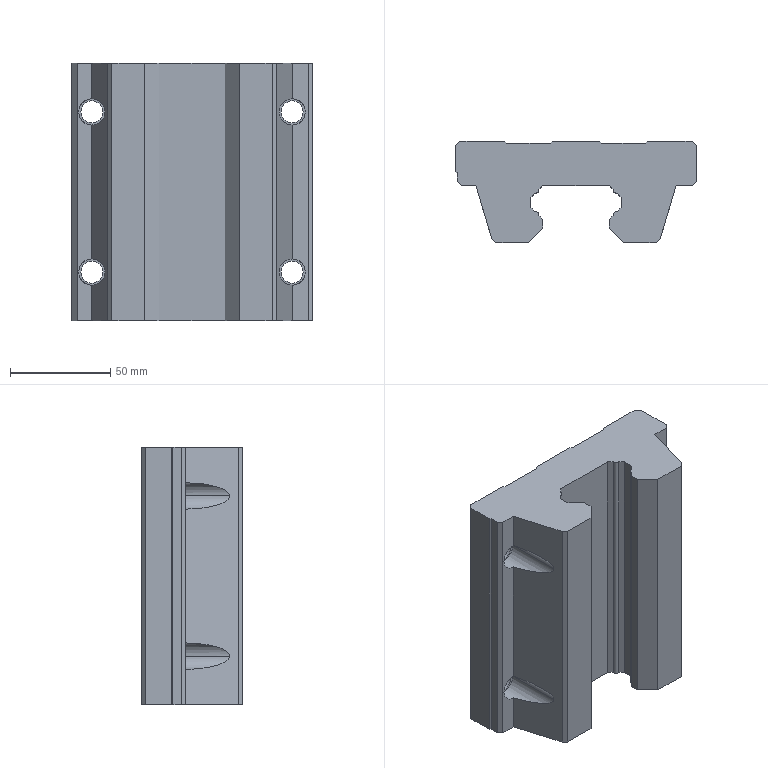Part | SolidWorks | features SplitBody 1 | 1 solid | 68 faces | box 120 x 50.5 x 128.8 mm | volume 512152 mm3 | plane 46 | cylinder 22 | commonest cylinder face diameters 11 x8 13.2 x8 3.924 x6